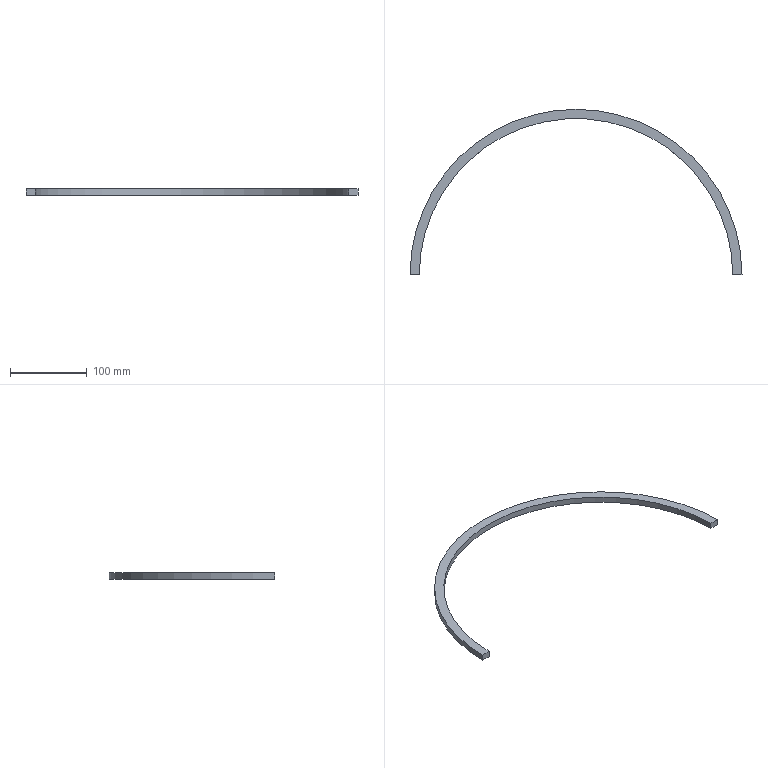Part | SolidWorks | features Extrusion 1 | 1 solid | 6 faces | box 431.995 x 215 x 8 mm | volume 63143 mm3 | plane 4 | cylinder 2 | commonest cylinder face diameters 408 x1 432 x1
STEP:
#1=CARTESIAN_POINT('',(435.998,1.,4.));
#2=VERTEX_POINT('',#1);
#3=CARTESIAN_POINT('',(4.002,1.,4.));
#4=VERTEX_POINT('',#3);
#5=CARTESIAN_POINT('',(220.,0.,4.));
#6=DIRECTION('',(0.,0.,1.));
#7=DIRECTION('',(1.,0.,0.));
#8=AXIS2_PLACEMENT_3D('',#5,#6,#7);
#9=CIRCLE('',#8,216.);
#10=EDGE_CURVE('',#2,#4,#9,.T.);
#11=ORIENTED_EDGE('',*,*,#10,.F.);
#12=CARTESIAN_POINT('',(435.998,1.,-4.));
#13=VERTEX_POINT('',#12);
#14=CARTESIAN_POINT('',(435.998,1.,-4.));
#15=DIRECTION('',(0.,0.,1.));
#16=VECTOR('',#15,1000.);
#17=LINE('',#14,#16);
#18=EDGE_CURVE('',#13,#2,#17,.T.);
#19=ORIENTED_EDGE('',*,*,#18,.F.);
#20=CARTESIAN_POINT('',(4.002,1.,-4.));
#21=VERTEX_POINT('',#20);
#22=CARTESIAN_POINT('',(220.,0.,-4.));
#23=DIRECTION('',(0.,0.,1.));
#24=DIRECTION('',(1.,0.,0.));
#25=AXIS2_PLACEMENT_3D('',#22,#23,#24);
#26=CIRCLE('',#25,216.);
#27=EDGE_CURVE('',#13,#21,#26,.T.);
#28=ORIENTED_EDGE('',*,*,#27,.T.);
#29=CARTESIAN_POINT('',(4.002,1.,-4.));
#30=DIRECTION('',(0.,0.,1.));
#31=VECTOR('',#30,1000.);
#32=LINE('',#29,#31);
#33=EDGE_CURVE('',#21,#4,#32,.T.);
#34=ORIENTED_EDGE('',*,*,#33,.T.);
#35=EDGE_LOOP('',(#11,#19,#28,#34));
#36=FACE_OUTER_BOUND('',#35,.T.);
#37=CARTESIAN_POINT('',(220.,0.,-4.));
#38=DIRECTION('',(0.,0.,1.));
#39=DIRECTION('',(1.,0.,0.));
#40=AXIS2_PLACEMENT_3D('',#37,#38,#39);
#41=CYLINDRICAL_SURFACE('',#40,216.);
#42=ADVANCED_FACE('',(#36),#41,.T.);
#43=CARTESIAN_POINT('',(423.998,1.,4.));
#44=VERTEX_POINT('',#43);
#45=CARTESIAN_POINT('',(423.998,1.,4.));
#46=DIRECTION('',(1.,0.,0.));
#47=VECTOR('',#46,1000.);
#48=LINE('',#45,#47);
#49=EDGE_CURVE('',#44,#2,#48,.T.);
#50=ORIENTED_EDGE('',*,*,#49,.F.);
#51=CARTESIAN_POINT('',(423.998,1.,-4.));
#52=VERTEX_POINT('',#51);
#53=CARTESIAN_POINT('',(423.998,1.,-4.));
#54=DIRECTION('',(0.,0.,1.));
#55=VECTOR('',#54,1000.);
#56=LINE('',#53,#55);
#57=EDGE_CURVE('',#52,#44,#56,.T.);
#58=ORIENTED_EDGE('',*,*,#57,.F.);
#59=CARTESIAN_POINT('',(423.998,1.,-4.));
#60=DIRECTION('',(1.,0.,0.));
#61=VECTOR('',#60,1000.);
#62=LINE('',#59,#61);
#63=EDGE_CURVE('',#52,#13,#62,.T.);
#64=ORIENTED_EDGE('',*,*,#63,.T.);
#65=ORIENTED_EDGE('',*,*,#18,.T.);
#66=EDGE_LOOP('',(#50,#58,#64,#65));
#67=FACE_OUTER_BOUND('',#66,.T.);
#68=CARTESIAN_POINT('',(423.998,1.,-4.));
#69=DIRECTION('',(0.,-1.,0.));
#70=DIRECTION('',(1.,0.,0.));
#71=AXIS2_PLACEMENT_3D('',#68,#69,#70);
#72=PLANE('',#71);
#73=ADVANCED_FACE('',(#67),#72,.T.);
#74=CARTESIAN_POINT('',(16.002,1.,4.));
#75=VERTEX_POINT('',#74);
#76=CARTESIAN_POINT('',(220.,0.,4.));
#77=DIRECTION('',(0.,0.,-1.));
#78=DIRECTION('',(-1.,0.,0.));
#79=AXIS2_PLACEMENT_3D('',#76,#77,#78);
#80=CIRCLE('',#79,204.);
#81=EDGE_CURVE('',#75,#44,#80,.T.);
#82=ORIENTED_EDGE('',*,*,#81,.F.);
#83=CARTESIAN_POINT('',(16.002,1.,-4.));
#84=VERTEX_POINT('',#83);
#85=CARTESIAN_POINT('',(16.002,1.,-4.));
#86=DIRECTION('',(0.,0.,1.));
#87=VECTOR('',#86,1000.);
#88=LINE('',#85,#87);
#89=EDGE_CURVE('',#84,#75,#88,.T.);
#90=ORIENTED_EDGE('',*,*,#89,.F.);
#91=CARTESIAN_POINT('',(220.,0.,-4.));
#92=DIRECTION('',(0.,0.,-1.));
#93=DIRECTION('',(-1.,0.,0.));
#94=AXIS2_PLACEMENT_3D('',#91,#92,#93);
#95=CIRCLE('',#94,204.);
#96=EDGE_CURVE('',#84,#52,#95,.T.);
#97=ORIENTED_EDGE('',*,*,#96,.T.);
#98=ORIENTED_EDGE('',*,*,#57,.T.);
#99=EDGE_LOOP('',(#82,#90,#97,#98));
#100=FACE_OUTER_BOUND('',#99,.T.);
#101=CARTESIAN_POINT('',(220.,0.,-4.));
#102=DIRECTION('',(0.,0.,1.));
#103=DIRECTION('',(1.,0.,0.));
#104=AXIS2_PLACEMENT_3D('',#101,#102,#103);
#105=CYLINDRICAL_SURFACE('',#104,204.);
#106=ADVANCED_FACE('',(#100),#105,.F.);
#107=CARTESIAN_POINT('',(4.002,1.,4.));
#108=DIRECTION('',(1.,0.,0.));
#109=VECTOR('',#108,1000.);
#110=LINE('',#107,#109);
#111=EDGE_CURVE('',#4,#75,#110,.T.);
#112=ORIENTED_EDGE('',*,*,#111,.F.);
#113=ORIENTED_EDGE('',*,*,#33,.F.);
#114=CARTESIAN_POINT('',(4.002,1.,-4.));
#115=DIRECTION('',(1.,0.,0.));
#116=VECTOR('',#115,1000.);
#117=LINE('',#114,#116);
#118=EDGE_CURVE('',#21,#84,#117,.T.);
#119=ORIENTED_EDGE('',*,*,#118,.T.);
#120=ORIENTED_EDGE('',*,*,#89,.T.);
#121=EDGE_LOOP('',(#112,#113,#119,#120));
#122=FACE_OUTER_BOUND('',#121,.T.);
#123=CARTESIAN_POINT('',(4.002,1.,-4.));
#124=DIRECTION('',(0.,-1.,0.));
#125=DIRECTION('',(1.,0.,0.));
#126=AXIS2_PLACEMENT_3D('',#123,#124,#125);
#127=PLANE('',#126);
#128=ADVANCED_FACE('',(#122),#127,.T.);
#129=ORIENTED_EDGE('',*,*,#27,.F.);
#130=ORIENTED_EDGE('',*,*,#63,.F.);
#131=ORIENTED_EDGE('',*,*,#96,.F.);
#132=ORIENTED_EDGE('',*,*,#118,.F.);
#133=EDGE_LOOP('',(#129,#130,#131,#132));
#134=FACE_OUTER_BOUND('',#133,.T.);
#135=CARTESIAN_POINT('',(220.,0.,-4.));
#136=DIRECTION('',(0.,0.,1.));
#137=DIRECTION('',(1.,0.,0.));
#138=AXIS2_PLACEMENT_3D('',#135,#136,#137);
#139=PLANE('',#138);
#140=ADVANCED_FACE('',(#134),#139,.F.);
#141=ORIENTED_EDGE('',*,*,#10,.T.);
#142=ORIENTED_EDGE('',*,*,#111,.T.);
#143=ORIENTED_EDGE('',*,*,#81,.T.);
#144=ORIENTED_EDGE('',*,*,#49,.T.);
#145=EDGE_LOOP('',(#141,#142,#143,#144));
#146=FACE_OUTER_BOUND('',#145,.T.);
#147=CARTESIAN_POINT('',(220.,0.,4.));
#148=DIRECTION('',(0.,0.,1.));
#149=DIRECTION('',(1.,0.,0.));
#150=AXIS2_PLACEMENT_3D('',#147,#148,#149);
#151=PLANE('',#150);
#152=ADVANCED_FACE('',(#146),#151,.T.);
#153=CLOSED_SHELL('',(#42,#73,#106,#128,#140,#152));
#154=MANIFOLD_SOLID_BREP('',#153);
#155=CARTESIAN_POINT('',(0.,0.,0.));
#156=DIRECTION('',(0.,0.,1.));
#157=DIRECTION('',(1.,0.,0.));
#158=AXIS2_PLACEMENT_3D('',#155,#156,#157);
#159=(LENGTH_UNIT()NAMED_UNIT(*)SI_UNIT(.MILLI.,.METRE.));
#160=UNCERTAINTY_MEASURE_WITH_UNIT(LENGTH_MEASURE(0.00001),#159,'','');
#161=(NAMED_UNIT(*)PLANE_ANGLE_UNIT()SI_UNIT($,.RADIAN.));
#162=(NAMED_UNIT(*)SI_UNIT($,.STERADIAN.)SOLID_ANGLE_UNIT());
#163=(GEOMETRIC_REPRESENTATION_CONTEXT(3)GLOBAL_UNCERTAINTY_ASSIGNED_CONTEXT((#160))GLOBAL_UNIT_ASSIGNED_CONTEXT((#159,#161,#162))REPRESENTATION_CONTEXT('',''));
#164=ADVANCED_BREP_SHAPE_REPRESENTATION('',(#154,#158),#163);